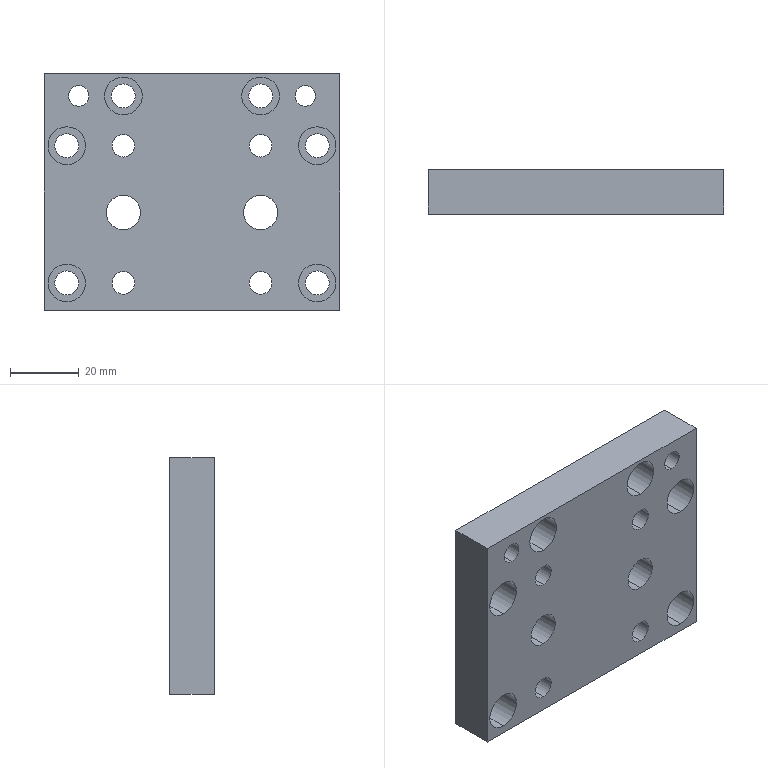Part | STEP file | OP10-118_cylinder base (1) | 1 solid | 64 faces | box 86 x 13 x 69 mm | volume 65313 mm3 | cylinder 48 | plane 16 | commonest cylinder face diameters 11 x20 7 x12 6.6 x8 6 x4 10 x4